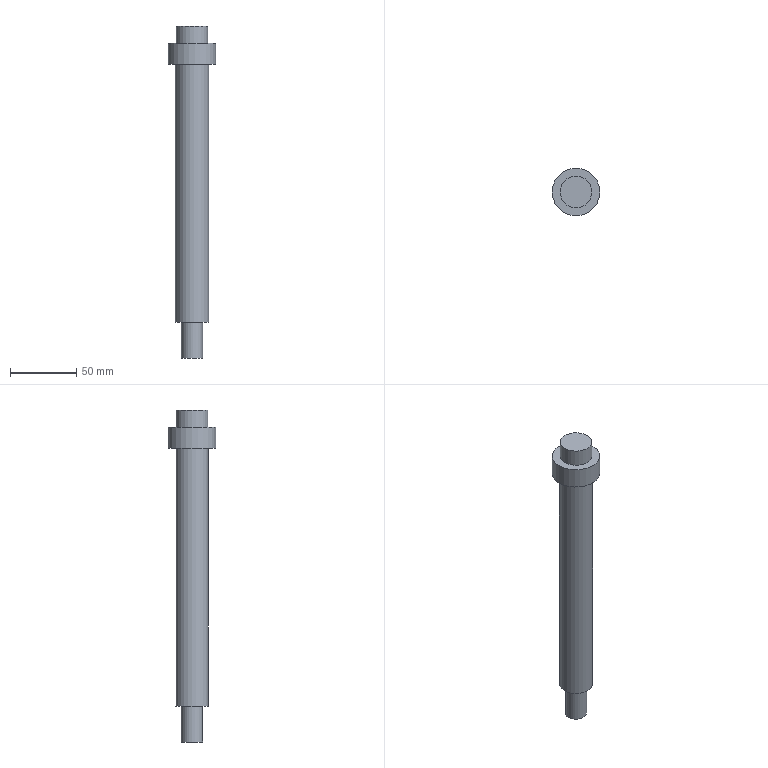Part | NX | features solid 2 | 1 solid | 9 faces | box 36 x 36 x 251 mm | volume 123316 mm3 | plane 5 | cylinder 4 | commonest cylinder face diameters 16 x1 24 x1 25 x1 36 x1
STEP:
#1=CARTESIAN_POINT('',(-8.,0.,130.));
#2=VERTEX_POINT('',#1);
#3=CARTESIAN_POINT('',(0.,0.,130.));
#4=DIRECTION('',(0.,0.,-1.));
#5=DIRECTION('',(-1.,0.,0.));
#6=AXIS2_PLACEMENT_3D('',#3,#4,#5);
#7=CIRCLE('',#6,8.);
#8=EDGE_CURVE('',#2,#2,#7,.T.);
#9=ORIENTED_EDGE('',*,*,#8,.F.);
#10=EDGE_LOOP('',(#9));
#11=FACE_BOUND('',#10,.T.);
#12=CARTESIAN_POINT('',(-12.5,0.,130.));
#13=VERTEX_POINT('',#12);
#14=CARTESIAN_POINT('',(0.,0.,130.));
#15=DIRECTION('',(0.,0.,-1.));
#16=DIRECTION('',(-1.,0.,0.));
#17=AXIS2_PLACEMENT_3D('',#14,#15,#16);
#18=CIRCLE('',#17,12.5);
#19=EDGE_CURVE('',#13,#13,#18,.F.);
#20=ORIENTED_EDGE('',*,*,#19,.F.);
#21=EDGE_LOOP('',(#20));
#22=FACE_BOUND('',#21,.T.);
#23=CARTESIAN_POINT('',(0.,0.,130.));
#24=DIRECTION('',(0.,0.,-1.));
#25=DIRECTION('',(-1.,0.,0.));
#26=AXIS2_PLACEMENT_3D('',#23,#24,#25);
#27=PLANE('',#26);
#28=ADVANCED_FACE('',(#11,#22),#27,.T.);
#29=CARTESIAN_POINT('',(-12.5,0.,325.));
#30=VERTEX_POINT('',#29);
#31=CARTESIAN_POINT('',(0.,0.,325.));
#32=DIRECTION('',(0.,0.,-1.));
#33=DIRECTION('',(-1.,0.,0.));
#34=AXIS2_PLACEMENT_3D('',#31,#32,#33);
#35=CIRCLE('',#34,12.5);
#36=EDGE_CURVE('',#30,#30,#35,.F.);
#37=ORIENTED_EDGE('',*,*,#36,.F.);
#38=EDGE_LOOP('',(#37));
#39=FACE_BOUND('',#38,.T.);
#40=ORIENTED_EDGE('',*,*,#19,.T.);
#41=EDGE_LOOP('',(#40));
#42=FACE_BOUND('',#41,.T.);
#43=CARTESIAN_POINT('',(0.,0.,110.));
#44=DIRECTION('',(0.,0.,1.));
#45=DIRECTION('',(1.,0.,0.));
#46=AXIS2_PLACEMENT_3D('',#43,#44,#45);
#47=CYLINDRICAL_SURFACE('',#46,12.5);
#48=ADVANCED_FACE('',(#39,#42),#47,.T.);
#49=CARTESIAN_POINT('',(-8.,0.,103.));
#50=VERTEX_POINT('',#49);
#51=CARTESIAN_POINT('',(0.,0.,103.));
#52=DIRECTION('',(0.,0.,-1.));
#53=DIRECTION('',(-1.,0.,0.));
#54=AXIS2_PLACEMENT_3D('',#51,#52,#53);
#55=CIRCLE('',#54,8.);
#56=EDGE_CURVE('',#50,#50,#55,.F.);
#57=ORIENTED_EDGE('',*,*,#56,.F.);
#58=EDGE_LOOP('',(#57));
#59=FACE_BOUND('',#58,.T.);
#60=CARTESIAN_POINT('',(0.,0.,103.));
#61=DIRECTION('',(0.,0.,-1.));
#62=DIRECTION('',(-1.,0.,0.));
#63=AXIS2_PLACEMENT_3D('',#60,#61,#62);
#64=PLANE('',#63);
#65=ADVANCED_FACE('',(#59),#64,.T.);
#66=ORIENTED_EDGE('',*,*,#56,.T.);
#67=EDGE_LOOP('',(#66));
#68=FACE_BOUND('',#67,.T.);
#69=ORIENTED_EDGE('',*,*,#8,.T.);
#70=EDGE_LOOP('',(#69));
#71=FACE_BOUND('',#70,.T.);
#72=CARTESIAN_POINT('',(0.,0.,110.));
#73=DIRECTION('',(0.,0.,-1.));
#74=DIRECTION('',(-1.,0.,0.));
#75=AXIS2_PLACEMENT_3D('',#72,#73,#74);
#76=CYLINDRICAL_SURFACE('',#75,8.);
#77=ADVANCED_FACE('',(#68,#71),#76,.T.);
#78=CARTESIAN_POINT('',(12.,0.,341.));
#79=VERTEX_POINT('',#78);
#80=CARTESIAN_POINT('',(0.,0.,341.));
#81=DIRECTION('',(0.,0.,1.));
#82=DIRECTION('',(1.,0.,0.));
#83=AXIS2_PLACEMENT_3D('',#80,#81,#82);
#84=CIRCLE('',#83,12.);
#85=EDGE_CURVE('',#79,#79,#84,.T.);
#86=ORIENTED_EDGE('',*,*,#85,.F.);
#87=EDGE_LOOP('',(#86));
#88=FACE_BOUND('',#87,.T.);
#89=CARTESIAN_POINT('',(18.,0.,341.));
#90=VERTEX_POINT('',#89);
#91=CARTESIAN_POINT('',(0.,0.,341.));
#92=DIRECTION('',(0.,0.,1.));
#93=DIRECTION('',(1.,0.,0.));
#94=AXIS2_PLACEMENT_3D('',#91,#92,#93);
#95=CIRCLE('',#94,18.);
#96=EDGE_CURVE('',#90,#90,#95,.F.);
#97=ORIENTED_EDGE('',*,*,#96,.F.);
#98=EDGE_LOOP('',(#97));
#99=FACE_BOUND('',#98,.T.);
#100=CARTESIAN_POINT('',(0.,0.,341.));
#101=DIRECTION('',(0.,0.,1.));
#102=DIRECTION('',(1.,0.,0.));
#103=AXIS2_PLACEMENT_3D('',#100,#101,#102);
#104=PLANE('',#103);
#105=ADVANCED_FACE('',(#88,#99),#104,.T.);
#106=ORIENTED_EDGE('',*,*,#36,.T.);
#107=EDGE_LOOP('',(#106));
#108=FACE_BOUND('',#107,.T.);
#109=CARTESIAN_POINT('',(-18.,0.,325.));
#110=VERTEX_POINT('',#109);
#111=CARTESIAN_POINT('',(0.,0.,325.));
#112=DIRECTION('',(0.,0.,-1.));
#113=DIRECTION('',(-1.,0.,0.));
#114=AXIS2_PLACEMENT_3D('',#111,#112,#113);
#115=CIRCLE('',#114,18.);
#116=EDGE_CURVE('',#110,#110,#115,.F.);
#117=ORIENTED_EDGE('',*,*,#116,.F.);
#118=EDGE_LOOP('',(#117));
#119=FACE_BOUND('',#118,.T.);
#120=CARTESIAN_POINT('',(0.,0.,325.));
#121=DIRECTION('',(0.,0.,-1.));
#122=DIRECTION('',(-1.,0.,0.));
#123=AXIS2_PLACEMENT_3D('',#120,#121,#122);
#124=PLANE('',#123);
#125=ADVANCED_FACE('',(#108,#119),#124,.T.);
#126=ORIENTED_EDGE('',*,*,#96,.T.);
#127=EDGE_LOOP('',(#126));
#128=FACE_BOUND('',#127,.T.);
#129=ORIENTED_EDGE('',*,*,#116,.T.);
#130=EDGE_LOOP('',(#129));
#131=FACE_BOUND('',#130,.T.);
#132=CARTESIAN_POINT('',(0.,0.,450.));
#133=DIRECTION('',(0.,0.,1.));
#134=DIRECTION('',(1.,0.,0.));
#135=AXIS2_PLACEMENT_3D('',#132,#133,#134);
#136=CYLINDRICAL_SURFACE('',#135,18.);
#137=ADVANCED_FACE('',(#128,#131),#136,.T.);
#138=CARTESIAN_POINT('',(12.,0.,354.));
#139=VERTEX_POINT('',#138);
#140=CARTESIAN_POINT('',(0.,0.,354.));
#141=DIRECTION('',(0.,0.,1.));
#142=DIRECTION('',(1.,0.,0.));
#143=AXIS2_PLACEMENT_3D('',#140,#141,#142);
#144=CIRCLE('',#143,12.);
#145=EDGE_CURVE('',#139,#139,#144,.F.);
#146=ORIENTED_EDGE('',*,*,#145,.F.);
#147=EDGE_LOOP('',(#146));
#148=FACE_BOUND('',#147,.T.);
#149=CARTESIAN_POINT('',(0.,0.,354.));
#150=DIRECTION('',(0.,0.,1.));
#151=DIRECTION('',(1.,0.,0.));
#152=AXIS2_PLACEMENT_3D('',#149,#150,#151);
#153=PLANE('',#152);
#154=ADVANCED_FACE('',(#148),#153,.T.);
#155=ORIENTED_EDGE('',*,*,#145,.T.);
#156=EDGE_LOOP('',(#155));
#157=FACE_BOUND('',#156,.T.);
#158=ORIENTED_EDGE('',*,*,#85,.T.);
#159=EDGE_LOOP('',(#158));
#160=FACE_BOUND('',#159,.T.);
#161=CARTESIAN_POINT('',(0.,0.,466.));
#162=DIRECTION('',(0.,0.,1.));
#163=DIRECTION('',(1.,0.,0.));
#164=AXIS2_PLACEMENT_3D('',#161,#162,#163);
#165=CYLINDRICAL_SURFACE('',#164,12.);
#166=ADVANCED_FACE('',(#157,#160),#165,.T.);
#167=CLOSED_SHELL('',(#28,#48,#65,#77,#105,#125,#137,#154,#166));
#168=MANIFOLD_SOLID_BREP('',#167);
#169=(LENGTH_UNIT()NAMED_UNIT(*)SI_UNIT(.MILLI.,.METRE.));
#170=UNCERTAINTY_MEASURE_WITH_UNIT(LENGTH_MEASURE(0.00001),#169,'','');
#171=(NAMED_UNIT(*)PLANE_ANGLE_UNIT()SI_UNIT($,.RADIAN.));
#172=(NAMED_UNIT(*)SI_UNIT($,.STERADIAN.)SOLID_ANGLE_UNIT());
#173=(GEOMETRIC_REPRESENTATION_CONTEXT(3)GLOBAL_UNCERTAINTY_ASSIGNED_CONTEXT((#170))GLOBAL_UNIT_ASSIGNED_CONTEXT((#169,#171,#172))REPRESENTATION_CONTEXT('',''));
#174=ADVANCED_BREP_SHAPE_REPRESENTATION('',(#168),#173);